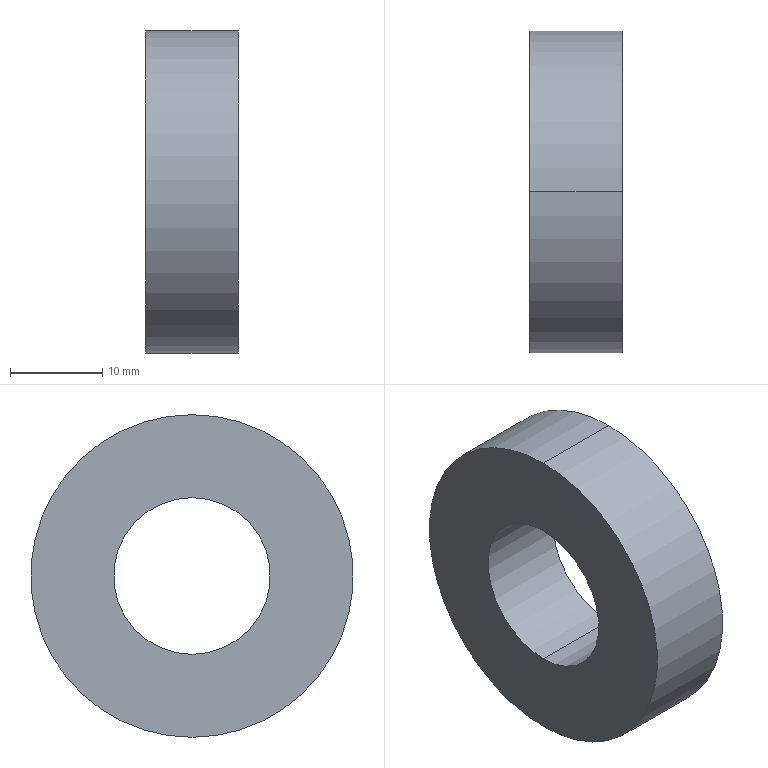Part | STEP file | PN_0022 (ZZ6003) | 1 solid | 6 faces | box 10 x 35 x 35 mm | volume 7351 mm3 | cylinder 4 | plane 2 | commonest cylinder face diameters 17 x2 35 x2
STEP:
#1=CARTESIAN_POINT('',(0.,0.,0.));
#2=DIRECTION('',(0.,0.,1.));
#3=DIRECTION('',(1.,0.,0.));
#4=AXIS2_PLACEMENT_3D('',#1,#2,#3);
#5=CARTESIAN_POINT('',(10.,0.,8.5));
#6=VERTEX_POINT('',#5);
#7=CARTESIAN_POINT('',(0.,0.,8.5));
#8=VERTEX_POINT('',#7);
#9=CARTESIAN_POINT('',(10.,0.,8.5));
#10=DIRECTION('',(-1.,0.,0.));
#11=VECTOR('',#10,1.);
#12=LINE('',#9,#11);
#13=CARTESIAN_POINT('',(10.,0.,0.));
#14=DIRECTION('',(-1.,0.,0.));
#15=DIRECTION('',(0.,0.,1.));
#16=AXIS2_PLACEMENT_3D('',#13,#14,#15);
#17=CYLINDRICAL_SURFACE('',#16,8.5);
#18=CARTESIAN_POINT('',(6.283,0.));
#19=DIRECTION('',(0.,1.));
#20=VECTOR('',#19,1.);
#21=LINE('',#18,#20);
#22=(GEOMETRIC_REPRESENTATION_CONTEXT(2)PARAMETRIC_REPRESENTATION_CONTEXT()REPRESENTATION_CONTEXT('',''));
#23=DEFINITIONAL_REPRESENTATION('',(#21),#22);
#24=PCURVE('',#17,#23);
#25=CARTESIAN_POINT('',(10.,0.,0.));
#26=DIRECTION('',(-1.,0.,0.));
#27=DIRECTION('',(0.,0.,1.));
#28=AXIS2_PLACEMENT_3D('',#25,#26,#27);
#29=CYLINDRICAL_SURFACE('',#28,8.5);
#30=CARTESIAN_POINT('',(0.,0.));
#31=DIRECTION('',(0.,1.));
#32=VECTOR('',#31,1.);
#33=LINE('',#30,#32);
#34=(GEOMETRIC_REPRESENTATION_CONTEXT(2)PARAMETRIC_REPRESENTATION_CONTEXT()REPRESENTATION_CONTEXT('',''));
#35=DEFINITIONAL_REPRESENTATION('',(#33),#34);
#36=PCURVE('',#29,#35);
#37=SURFACE_CURVE('',#12,(#24,#36),.PCURVE_S1.);
#38=EDGE_CURVE('',#6,#8,#37,.T.);
#39=ORIENTED_EDGE('',*,*,#38,.T.);
#40=CARTESIAN_POINT('',(0.,0.,-8.5));
#41=VERTEX_POINT('',#40);
#42=CARTESIAN_POINT('',(0.,0.,0.));
#43=DIRECTION('',(1.,0.,0.));
#44=DIRECTION('',(0.,0.,-1.));
#45=AXIS2_PLACEMENT_3D('',#42,#43,#44);
#46=CIRCLE('',#45,8.5);
#47=CARTESIAN_POINT('',(9.425,10.));
#48=DIRECTION('',(-1.,0.));
#49=VECTOR('',#48,1.);
#50=LINE('',#47,#49);
#51=(GEOMETRIC_REPRESENTATION_CONTEXT(2)PARAMETRIC_REPRESENTATION_CONTEXT()REPRESENTATION_CONTEXT('',''));
#52=DEFINITIONAL_REPRESENTATION('',(#50),#51);
#53=PCURVE('',#17,#52);
#54=CARTESIAN_POINT('',(0.,0.,0.));
#55=DIRECTION('',(1.,0.,0.));
#56=DIRECTION('',(0.,0.,-1.));
#57=AXIS2_PLACEMENT_3D('',#54,#55,#56);
#58=PLANE('',#57);
#59=CARTESIAN_POINT('',(0.,0.));
#60=DIRECTION('',(1.,0.));
#61=AXIS2_PLACEMENT_2D('',#59,#60);
#62=CIRCLE('',#61,8.5);
#63=(GEOMETRIC_REPRESENTATION_CONTEXT(2)PARAMETRIC_REPRESENTATION_CONTEXT()REPRESENTATION_CONTEXT('',''));
#64=DEFINITIONAL_REPRESENTATION('',(#62),#63);
#65=PCURVE('',#58,#64);
#66=SURFACE_CURVE('',#46,(#53,#65),.PCURVE_S1.);
#67=EDGE_CURVE('',#8,#41,#66,.T.);
#68=ORIENTED_EDGE('',*,*,#67,.T.);
#69=CARTESIAN_POINT('',(10.,0.,-8.5));
#70=VERTEX_POINT('',#69);
#71=CARTESIAN_POINT('',(10.,0.,-8.5));
#72=DIRECTION('',(-1.,0.,0.));
#73=VECTOR('',#72,1.);
#74=LINE('',#71,#73);
#75=CARTESIAN_POINT('',(3.142,0.));
#76=DIRECTION('',(0.,1.));
#77=VECTOR('',#76,1.);
#78=LINE('',#75,#77);
#79=(GEOMETRIC_REPRESENTATION_CONTEXT(2)PARAMETRIC_REPRESENTATION_CONTEXT()REPRESENTATION_CONTEXT('',''));
#80=DEFINITIONAL_REPRESENTATION('',(#78),#79);
#81=PCURVE('',#17,#80);
#82=CARTESIAN_POINT('',(3.142,0.));
#83=DIRECTION('',(0.,1.));
#84=VECTOR('',#83,1.);
#85=LINE('',#82,#84);
#86=(GEOMETRIC_REPRESENTATION_CONTEXT(2)PARAMETRIC_REPRESENTATION_CONTEXT()REPRESENTATION_CONTEXT('',''));
#87=DEFINITIONAL_REPRESENTATION('',(#85),#86);
#88=PCURVE('',#29,#87);
#89=SURFACE_CURVE('',#74,(#81,#88),.PCURVE_S1.);
#90=EDGE_CURVE('',#70,#41,#89,.T.);
#91=ORIENTED_EDGE('',*,*,#90,.F.);
#92=CARTESIAN_POINT('',(10.,0.,0.));
#93=DIRECTION('',(1.,0.,0.));
#94=DIRECTION('',(0.,0.,-1.));
#95=AXIS2_PLACEMENT_3D('',#92,#93,#94);
#96=CIRCLE('',#95,8.5);
#97=CARTESIAN_POINT('',(9.425,0.));
#98=DIRECTION('',(-1.,0.));
#99=VECTOR('',#98,1.);
#100=LINE('',#97,#99);
#101=(GEOMETRIC_REPRESENTATION_CONTEXT(2)PARAMETRIC_REPRESENTATION_CONTEXT()REPRESENTATION_CONTEXT('',''));
#102=DEFINITIONAL_REPRESENTATION('',(#100),#101);
#103=PCURVE('',#17,#102);
#104=CARTESIAN_POINT('',(10.,0.,0.));
#105=DIRECTION('',(1.,0.,0.));
#106=DIRECTION('',(0.,0.,-1.));
#107=AXIS2_PLACEMENT_3D('',#104,#105,#106);
#108=PLANE('',#107);
#109=CARTESIAN_POINT('',(0.,0.));
#110=DIRECTION('',(1.,0.));
#111=AXIS2_PLACEMENT_2D('',#109,#110);
#112=CIRCLE('',#111,8.5);
#113=(GEOMETRIC_REPRESENTATION_CONTEXT(2)PARAMETRIC_REPRESENTATION_CONTEXT()REPRESENTATION_CONTEXT('',''));
#114=DEFINITIONAL_REPRESENTATION('',(#112),#113);
#115=PCURVE('',#108,#114);
#116=SURFACE_CURVE('',#96,(#103,#115),.PCURVE_S1.);
#117=EDGE_CURVE('',#6,#70,#116,.T.);
#118=ORIENTED_EDGE('',*,*,#117,.F.);
#119=EDGE_LOOP('',(#39,#68,#91,#118));
#120=FACE_BOUND('',#119,.F.);
#121=ADVANCED_FACE('',(#120),#17,.F.);
#122=CARTESIAN_POINT('',(10.,0.,-17.5));
#123=VERTEX_POINT('',#122);
#124=CARTESIAN_POINT('',(10.,0.,17.5));
#125=VERTEX_POINT('',#124);
#126=CARTESIAN_POINT('',(10.,0.,0.));
#127=DIRECTION('',(1.,0.,0.));
#128=DIRECTION('',(0.,0.,-1.));
#129=AXIS2_PLACEMENT_3D('',#126,#127,#128);
#130=CIRCLE('',#129,17.5);
#131=CARTESIAN_POINT('',(10.,0.,0.));
#132=DIRECTION('',(-1.,0.,0.));
#133=DIRECTION('',(0.,0.,1.));
#134=AXIS2_PLACEMENT_3D('',#131,#132,#133);
#135=CYLINDRICAL_SURFACE('',#134,17.5);
#136=CARTESIAN_POINT('',(3.142,0.));
#137=DIRECTION('',(-1.,0.));
#138=VECTOR('',#137,1.);
#139=LINE('',#136,#138);
#140=(GEOMETRIC_REPRESENTATION_CONTEXT(2)PARAMETRIC_REPRESENTATION_CONTEXT()REPRESENTATION_CONTEXT('',''));
#141=DEFINITIONAL_REPRESENTATION('',(#139),#140);
#142=PCURVE('',#135,#141);
#143=CARTESIAN_POINT('',(0.,0.));
#144=DIRECTION('',(1.,0.));
#145=AXIS2_PLACEMENT_2D('',#143,#144);
#146=CIRCLE('',#145,17.5);
#147=(GEOMETRIC_REPRESENTATION_CONTEXT(2)PARAMETRIC_REPRESENTATION_CONTEXT()REPRESENTATION_CONTEXT('',''));
#148=DEFINITIONAL_REPRESENTATION('',(#146),#147);
#149=PCURVE('',#108,#148);
#150=SURFACE_CURVE('',#130,(#142,#149),.PCURVE_S1.);
#151=EDGE_CURVE('',#123,#125,#150,.T.);
#152=ORIENTED_EDGE('',*,*,#151,.F.);
#153=CARTESIAN_POINT('',(0.,0.,-17.5));
#154=VERTEX_POINT('',#153);
#155=CARTESIAN_POINT('',(10.,0.,-17.5));
#156=DIRECTION('',(-1.,0.,0.));
#157=VECTOR('',#156,1.);
#158=LINE('',#155,#157);
#159=CARTESIAN_POINT('',(3.142,0.));
#160=DIRECTION('',(0.,1.));
#161=VECTOR('',#160,1.);
#162=LINE('',#159,#161);
#163=(GEOMETRIC_REPRESENTATION_CONTEXT(2)PARAMETRIC_REPRESENTATION_CONTEXT()REPRESENTATION_CONTEXT('',''));
#164=DEFINITIONAL_REPRESENTATION('',(#162),#163);
#165=PCURVE('',#135,#164);
#166=CARTESIAN_POINT('',(10.,0.,0.));
#167=DIRECTION('',(-1.,0.,0.));
#168=DIRECTION('',(0.,0.,1.));
#169=AXIS2_PLACEMENT_3D('',#166,#167,#168);
#170=CYLINDRICAL_SURFACE('',#169,17.5);
#171=CARTESIAN_POINT('',(3.142,0.));
#172=DIRECTION('',(0.,1.));
#173=VECTOR('',#172,1.);
#174=LINE('',#171,#173);
#175=(GEOMETRIC_REPRESENTATION_CONTEXT(2)PARAMETRIC_REPRESENTATION_CONTEXT()REPRESENTATION_CONTEXT('',''));
#176=DEFINITIONAL_REPRESENTATION('',(#174),#175);
#177=PCURVE('',#170,#176);
#178=SURFACE_CURVE('',#158,(#165,#177),.PCURVE_S1.);
#179=EDGE_CURVE('',#123,#154,#178,.T.);
#180=ORIENTED_EDGE('',*,*,#179,.T.);
#181=CARTESIAN_POINT('',(0.,0.,17.5));
#182=VERTEX_POINT('',#181);
#183=CARTESIAN_POINT('',(0.,0.,0.));
#184=DIRECTION('',(1.,0.,0.));
#185=DIRECTION('',(0.,0.,-1.));
#186=AXIS2_PLACEMENT_3D('',#183,#184,#185);
#187=CIRCLE('',#186,17.5);
#188=CARTESIAN_POINT('',(3.142,10.));
#189=DIRECTION('',(-1.,0.));
#190=VECTOR('',#189,1.);
#191=LINE('',#188,#190);
#192=(GEOMETRIC_REPRESENTATION_CONTEXT(2)PARAMETRIC_REPRESENTATION_CONTEXT()REPRESENTATION_CONTEXT('',''));
#193=DEFINITIONAL_REPRESENTATION('',(#191),#192);
#194=PCURVE('',#135,#193);
#195=CARTESIAN_POINT('',(0.,0.));
#196=DIRECTION('',(1.,0.));
#197=AXIS2_PLACEMENT_2D('',#195,#196);
#198=CIRCLE('',#197,17.5);
#199=(GEOMETRIC_REPRESENTATION_CONTEXT(2)PARAMETRIC_REPRESENTATION_CONTEXT()REPRESENTATION_CONTEXT('',''));
#200=DEFINITIONAL_REPRESENTATION('',(#198),#199);
#201=PCURVE('',#58,#200);
#202=SURFACE_CURVE('',#187,(#194,#201),.PCURVE_S1.);
#203=EDGE_CURVE('',#154,#182,#202,.T.);
#204=ORIENTED_EDGE('',*,*,#203,.T.);
#205=CARTESIAN_POINT('',(10.,0.,17.5));
#206=DIRECTION('',(-1.,0.,0.));
#207=VECTOR('',#206,1.);
#208=LINE('',#205,#207);
#209=CARTESIAN_POINT('',(0.,0.));
#210=DIRECTION('',(0.,1.));
#211=VECTOR('',#210,1.);
#212=LINE('',#209,#211);
#213=(GEOMETRIC_REPRESENTATION_CONTEXT(2)PARAMETRIC_REPRESENTATION_CONTEXT()REPRESENTATION_CONTEXT('',''));
#214=DEFINITIONAL_REPRESENTATION('',(#212),#213);
#215=PCURVE('',#135,#214);
#216=CARTESIAN_POINT('',(6.283,0.));
#217=DIRECTION('',(0.,1.));
#218=VECTOR('',#217,1.);
#219=LINE('',#216,#218);
#220=(GEOMETRIC_REPRESENTATION_CONTEXT(2)PARAMETRIC_REPRESENTATION_CONTEXT()REPRESENTATION_CONTEXT('',''));
#221=DEFINITIONAL_REPRESENTATION('',(#219),#220);
#222=PCURVE('',#170,#221);
#223=SURFACE_CURVE('',#208,(#215,#222),.PCURVE_S1.);
#224=EDGE_CURVE('',#125,#182,#223,.T.);
#225=ORIENTED_EDGE('',*,*,#224,.F.);
#226=EDGE_LOOP('',(#152,#180,#204,#225));
#227=FACE_BOUND('',#226,.T.);
#228=ADVANCED_FACE('',(#227),#135,.T.);
#229=CARTESIAN_POINT('',(10.,0.,0.));
#230=DIRECTION('',(1.,0.,0.));
#231=DIRECTION('',(0.,0.,-1.));
#232=AXIS2_PLACEMENT_3D('',#229,#230,#231);
#233=CIRCLE('',#232,17.5);
#234=CARTESIAN_POINT('',(0.,0.));
#235=DIRECTION('',(1.,0.));
#236=AXIS2_PLACEMENT_2D('',#234,#235);
#237=CIRCLE('',#236,17.5);
#238=(GEOMETRIC_REPRESENTATION_CONTEXT(2)PARAMETRIC_REPRESENTATION_CONTEXT()REPRESENTATION_CONTEXT('',''));
#239=DEFINITIONAL_REPRESENTATION('',(#237),#238);
#240=PCURVE('',#108,#239);
#241=CARTESIAN_POINT('',(9.425,0.));
#242=DIRECTION('',(-1.,0.));
#243=VECTOR('',#242,1.);
#244=LINE('',#241,#243);
#245=(GEOMETRIC_REPRESENTATION_CONTEXT(2)PARAMETRIC_REPRESENTATION_CONTEXT()REPRESENTATION_CONTEXT('',''));
#246=DEFINITIONAL_REPRESENTATION('',(#244),#245);
#247=PCURVE('',#170,#246);
#248=SURFACE_CURVE('',#233,(#240,#247),.PCURVE_S1.);
#249=EDGE_CURVE('',#125,#123,#248,.T.);
#250=ORIENTED_EDGE('',*,*,#249,.T.);
#251=ORIENTED_EDGE('',*,*,#151,.T.);
#252=EDGE_LOOP('',(#250,#251));
#253=FACE_BOUND('',#252,.T.);
#254=ORIENTED_EDGE('',*,*,#117,.F.);
#255=CARTESIAN_POINT('',(10.,0.,0.));
#256=DIRECTION('',(1.,0.,0.));
#257=DIRECTION('',(0.,0.,-1.));
#258=AXIS2_PLACEMENT_3D('',#255,#256,#257);
#259=CIRCLE('',#258,8.5);
#260=CARTESIAN_POINT('',(0.,0.));
#261=DIRECTION('',(1.,0.));
#262=AXIS2_PLACEMENT_2D('',#260,#261);
#263=CIRCLE('',#262,8.5);
#264=(GEOMETRIC_REPRESENTATION_CONTEXT(2)PARAMETRIC_REPRESENTATION_CONTEXT()REPRESENTATION_CONTEXT('',''));
#265=DEFINITIONAL_REPRESENTATION('',(#263),#264);
#266=PCURVE('',#108,#265);
#267=CARTESIAN_POINT('',(3.142,0.));
#268=DIRECTION('',(-1.,0.));
#269=VECTOR('',#268,1.);
#270=LINE('',#267,#269);
#271=(GEOMETRIC_REPRESENTATION_CONTEXT(2)PARAMETRIC_REPRESENTATION_CONTEXT()REPRESENTATION_CONTEXT('',''));
#272=DEFINITIONAL_REPRESENTATION('',(#270),#271);
#273=PCURVE('',#29,#272);
#274=SURFACE_CURVE('',#259,(#266,#273),.PCURVE_S1.);
#275=EDGE_CURVE('',#70,#6,#274,.T.);
#276=ORIENTED_EDGE('',*,*,#275,.F.);
#277=EDGE_LOOP('',(#254,#276));
#278=FACE_BOUND('',#277,.T.);
#279=ADVANCED_FACE('',(#253,#278),#108,.T.);
#280=CARTESIAN_POINT('',(0.,0.,0.));
#281=DIRECTION('',(1.,0.,0.));
#282=DIRECTION('',(0.,0.,-1.));
#283=AXIS2_PLACEMENT_3D('',#280,#281,#282);
#284=CIRCLE('',#283,17.5);
#285=CARTESIAN_POINT('',(0.,0.));
#286=DIRECTION('',(1.,0.));
#287=AXIS2_PLACEMENT_2D('',#285,#286);
#288=CIRCLE('',#287,17.5);
#289=(GEOMETRIC_REPRESENTATION_CONTEXT(2)PARAMETRIC_REPRESENTATION_CONTEXT()REPRESENTATION_CONTEXT('',''));
#290=DEFINITIONAL_REPRESENTATION('',(#288),#289);
#291=PCURVE('',#58,#290);
#292=CARTESIAN_POINT('',(9.425,10.));
#293=DIRECTION('',(-1.,0.));
#294=VECTOR('',#293,1.);
#295=LINE('',#292,#294);
#296=(GEOMETRIC_REPRESENTATION_CONTEXT(2)PARAMETRIC_REPRESENTATION_CONTEXT()REPRESENTATION_CONTEXT('',''));
#297=DEFINITIONAL_REPRESENTATION('',(#295),#296);
#298=PCURVE('',#170,#297);
#299=SURFACE_CURVE('',#284,(#291,#298),.PCURVE_S1.);
#300=EDGE_CURVE('',#182,#154,#299,.T.);
#301=ORIENTED_EDGE('',*,*,#300,.F.);
#302=ORIENTED_EDGE('',*,*,#203,.F.);
#303=EDGE_LOOP('',(#301,#302));
#304=FACE_BOUND('',#303,.T.);
#305=ORIENTED_EDGE('',*,*,#67,.T.);
#306=CARTESIAN_POINT('',(0.,0.,0.));
#307=DIRECTION('',(1.,0.,0.));
#308=DIRECTION('',(0.,0.,-1.));
#309=AXIS2_PLACEMENT_3D('',#306,#307,#308);
#310=CIRCLE('',#309,8.5);
#311=CARTESIAN_POINT('',(0.,0.));
#312=DIRECTION('',(1.,0.));
#313=AXIS2_PLACEMENT_2D('',#311,#312);
#314=CIRCLE('',#313,8.5);
#315=(GEOMETRIC_REPRESENTATION_CONTEXT(2)PARAMETRIC_REPRESENTATION_CONTEXT()REPRESENTATION_CONTEXT('',''));
#316=DEFINITIONAL_REPRESENTATION('',(#314),#315);
#317=PCURVE('',#58,#316);
#318=CARTESIAN_POINT('',(3.142,10.));
#319=DIRECTION('',(-1.,0.));
#320=VECTOR('',#319,1.);
#321=LINE('',#318,#320);
#322=(GEOMETRIC_REPRESENTATION_CONTEXT(2)PARAMETRIC_REPRESENTATION_CONTEXT()REPRESENTATION_CONTEXT('',''));
#323=DEFINITIONAL_REPRESENTATION('',(#321),#322);
#324=PCURVE('',#29,#323);
#325=SURFACE_CURVE('',#310,(#317,#324),.PCURVE_S1.);
#326=EDGE_CURVE('',#41,#8,#325,.T.);
#327=ORIENTED_EDGE('',*,*,#326,.T.);
#328=EDGE_LOOP('',(#305,#327));
#329=FACE_BOUND('',#328,.T.);
#330=ADVANCED_FACE('',(#304,#329),#58,.F.);
#331=ORIENTED_EDGE('',*,*,#179,.F.);
#332=ORIENTED_EDGE('',*,*,#249,.F.);
#333=ORIENTED_EDGE('',*,*,#224,.T.);
#334=ORIENTED_EDGE('',*,*,#300,.T.);
#335=EDGE_LOOP('',(#331,#332,#333,#334));
#336=FACE_BOUND('',#335,.T.);
#337=ADVANCED_FACE('',(#336),#170,.T.);
#338=ORIENTED_EDGE('',*,*,#326,.T.);
#339=ORIENTED_EDGE('',*,*,#38,.F.);
#340=ORIENTED_EDGE('',*,*,#275,.F.);
#341=ORIENTED_EDGE('',*,*,#90,.T.);
#342=EDGE_LOOP('',(#338,#339,#340,#341));
#343=FACE_BOUND('',#342,.F.);
#344=ADVANCED_FACE('',(#343),#29,.F.);
#345=CLOSED_SHELL('',(#121,#228,#279,#330,#337,#344));
#346=MANIFOLD_SOLID_BREP('',#345);
#347=(LENGTH_UNIT()NAMED_UNIT(*)SI_UNIT(.MILLI.,.METRE.));
#348=UNCERTAINTY_MEASURE_WITH_UNIT(LENGTH_MEASURE(0.0000001),#347,'','');
#349=(NAMED_UNIT(*)PLANE_ANGLE_UNIT()SI_UNIT($,.RADIAN.));
#350=(NAMED_UNIT(*)SI_UNIT($,.STERADIAN.)SOLID_ANGLE_UNIT());
#351=(GEOMETRIC_REPRESENTATION_CONTEXT(3)GLOBAL_UNCERTAINTY_ASSIGNED_CONTEXT((#348))GLOBAL_UNIT_ASSIGNED_CONTEXT((#347,#349,#350))REPRESENTATION_CONTEXT('',''));
#352=ADVANCED_BREP_SHAPE_REPRESENTATION('',(#4,#346),#351);